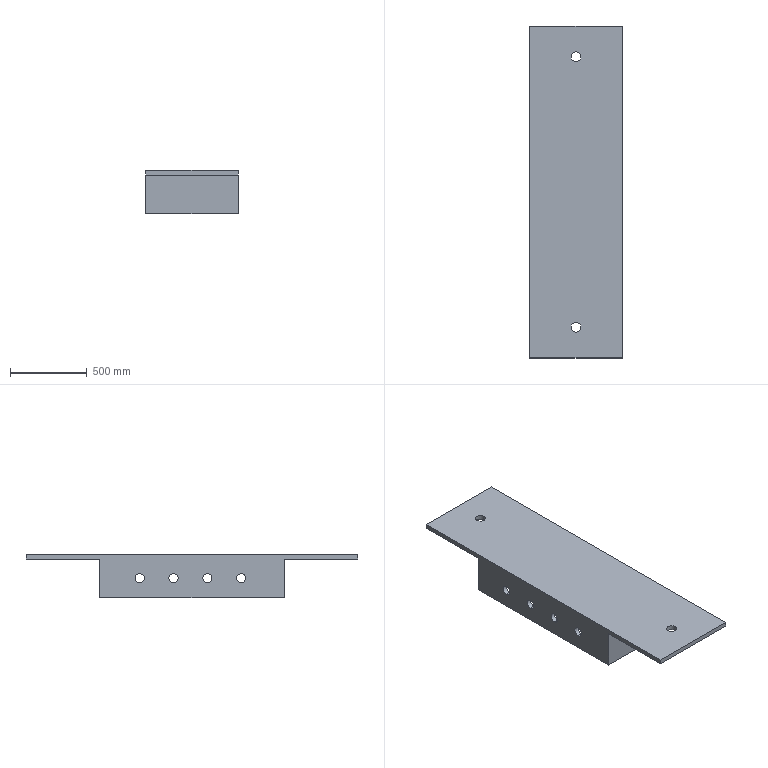Part | SolidWorks | features ICE 6, LPattern 5, Extrusion 1 | 1 solid | 71 faces | box 600 x 2160 x 280 mm | volume 64089547 mm3 | cylinder 44 | plane 27 | commonest cylinder face diameters 10 x24 60 x16 64 x4